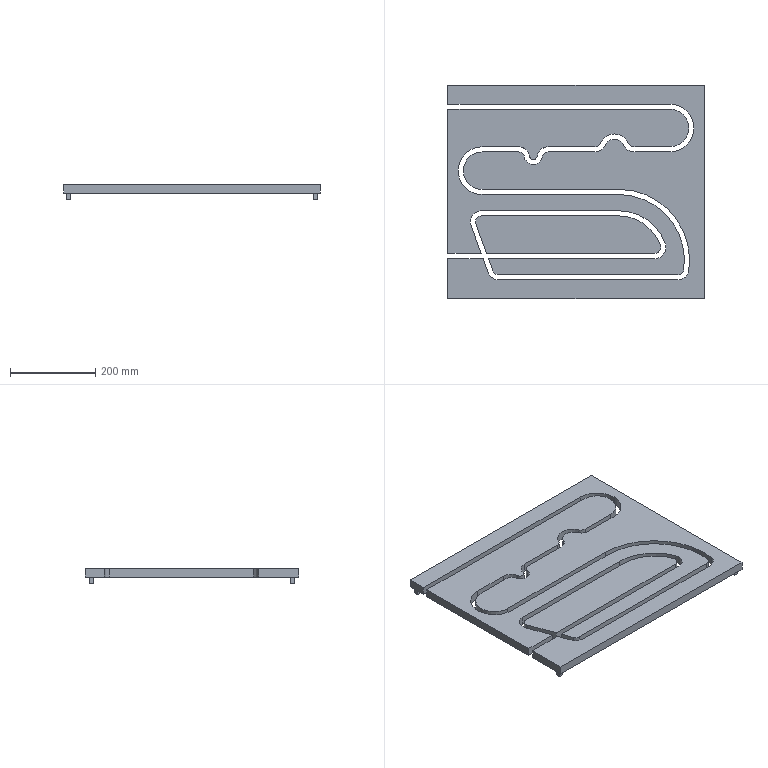Part | SolidWorks | features ICE 4, CutThin 2, MirrorPattern 2, Extrusion 1 | 3 solids | 84 faces | box 600 x 500 x 35 mm | volume 5161469 mm3 | plane 54 | cylinder 30 | commonest cylinder face diameters 28 x8 52 x8 88 x3 112 x3 18 x1 42 x1